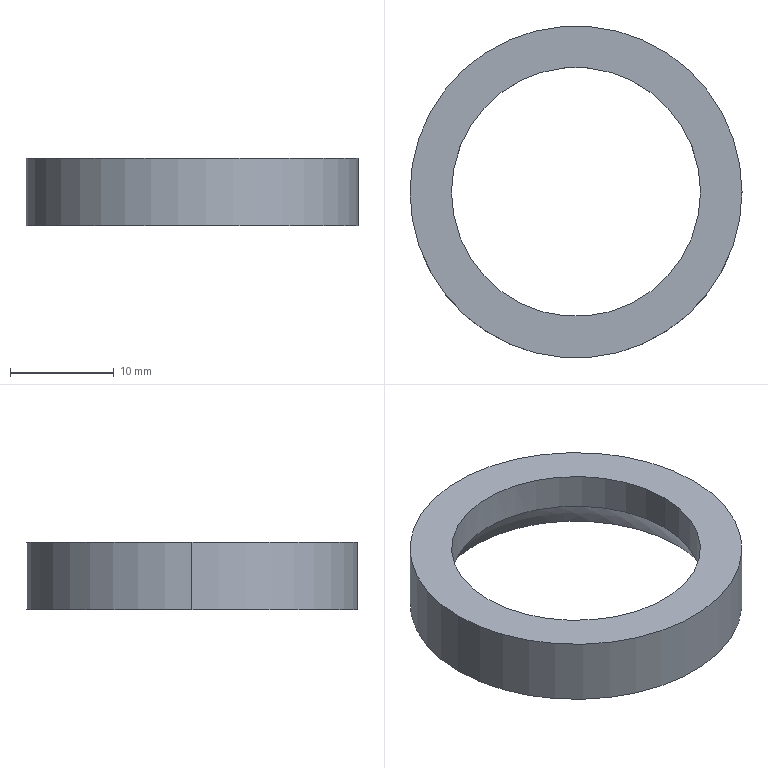Part | SolidWorks | features BaseBody 1 | 1 solid | 7 faces | box 32 x 32 x 6.5 mm | volume 2061 mm3 | cylinder 4 | plane 2 | spline 1 | commonest cylinder face diameters 24 x2 32 x2
STEP:
#1=CARTESIAN_POINT('',(16.,0.,0.));
#2=VERTEX_POINT('',#1);
#3=CARTESIAN_POINT('',(-16.,0.,0.));
#4=VERTEX_POINT('',#3);
#5=CARTESIAN_POINT('',(0.,0.,0.));
#6=DIRECTION('',(0.,0.,1.));
#7=DIRECTION('',(1.,0.,0.));
#8=AXIS2_PLACEMENT_3D('',#5,#6,#7);
#9=CIRCLE('',#8,16.);
#10=EDGE_CURVE('',#2,#4,#9,.T.);
#11=ORIENTED_EDGE('',*,*,#10,.T.);
#12=CARTESIAN_POINT('',(-16.,0.,6.5));
#13=VERTEX_POINT('',#12);
#14=CARTESIAN_POINT('',(-16.,0.,0.));
#15=DIRECTION('',(0.,0.,1.));
#16=VECTOR('',#15,1000.);
#17=LINE('',#14,#16);
#18=EDGE_CURVE('',#4,#13,#17,.T.);
#19=ORIENTED_EDGE('',*,*,#18,.T.);
#20=CARTESIAN_POINT('',(16.,0.,6.5));
#21=VERTEX_POINT('',#20);
#22=CARTESIAN_POINT('',(0.,0.,6.5));
#23=DIRECTION('',(0.,0.,-1.));
#24=DIRECTION('',(1.,0.,0.));
#25=AXIS2_PLACEMENT_3D('',#22,#23,#24);
#26=CIRCLE('',#25,16.);
#27=EDGE_CURVE('',#13,#21,#26,.T.);
#28=ORIENTED_EDGE('',*,*,#27,.T.);
#29=CARTESIAN_POINT('',(16.,0.,0.));
#30=DIRECTION('',(0.,0.,1.));
#31=VECTOR('',#30,1000.);
#32=LINE('',#29,#31);
#33=EDGE_CURVE('',#2,#21,#32,.T.);
#34=ORIENTED_EDGE('',*,*,#33,.F.);
#35=EDGE_LOOP('',(#11,#19,#28,#34));
#36=FACE_OUTER_BOUND('',#35,.T.);
#37=CARTESIAN_POINT('',(0.,0.,0.));
#38=DIRECTION('',(0.,0.,1.));
#39=DIRECTION('',(1.,0.,0.));
#40=AXIS2_PLACEMENT_3D('',#37,#38,#39);
#41=CYLINDRICAL_SURFACE('',#40,16.);
#42=ADVANCED_FACE('',(#36),#41,.T.);
#43=CARTESIAN_POINT('',(12.,0.,3.));
#44=VERTEX_POINT('',#43);
#45=CARTESIAN_POINT('',(-12.,0.,3.));
#46=VERTEX_POINT('',#45);
#47=CARTESIAN_POINT('',(0.,0.,3.));
#48=DIRECTION('',(0.,0.,-1.));
#49=DIRECTION('',(1.,0.,0.));
#50=AXIS2_PLACEMENT_3D('',#47,#48,#49);
#51=CIRCLE('',#50,12.);
#52=EDGE_CURVE('',#44,#46,#51,.T.);
#53=ORIENTED_EDGE('',*,*,#52,.T.);
#54=CARTESIAN_POINT('',(-12.,0.,6.5));
#55=VERTEX_POINT('',#54);
#56=CARTESIAN_POINT('',(-12.,0.,0.));
#57=DIRECTION('',(0.,0.,1.));
#58=VECTOR('',#57,1000.);
#59=LINE('',#56,#58);
#60=EDGE_CURVE('',#46,#55,#59,.T.);
#61=ORIENTED_EDGE('',*,*,#60,.T.);
#62=CARTESIAN_POINT('',(12.,0.,6.5));
#63=VERTEX_POINT('',#62);
#64=CARTESIAN_POINT('',(0.,0.,6.5));
#65=DIRECTION('',(0.,0.,-1.));
#66=DIRECTION('',(1.,0.,0.));
#67=AXIS2_PLACEMENT_3D('',#64,#65,#66);
#68=CIRCLE('',#67,12.);
#69=EDGE_CURVE('',#63,#55,#68,.T.);
#70=ORIENTED_EDGE('',*,*,#69,.F.);
#71=CARTESIAN_POINT('',(12.,0.,0.));
#72=DIRECTION('',(0.,0.,1.));
#73=VECTOR('',#72,1000.);
#74=LINE('',#71,#73);
#75=EDGE_CURVE('',#44,#63,#74,.T.);
#76=ORIENTED_EDGE('',*,*,#75,.F.);
#77=EDGE_LOOP('',(#53,#61,#70,#76));
#78=FACE_OUTER_BOUND('',#77,.T.);
#79=CARTESIAN_POINT('',(0.,0.,0.));
#80=DIRECTION('',(0.,0.,1.));
#81=DIRECTION('',(1.,0.,0.));
#82=AXIS2_PLACEMENT_3D('',#79,#80,#81);
#83=CYLINDRICAL_SURFACE('',#82,12.);
#84=ADVANCED_FACE('',(#78),#83,.F.);
#85=ORIENTED_EDGE('',*,*,#18,.F.);
#86=CARTESIAN_POINT('',(0.,0.,0.));
#87=DIRECTION('',(0.,0.,1.));
#88=DIRECTION('',(1.,0.,0.));
#89=AXIS2_PLACEMENT_3D('',#86,#87,#88);
#90=CIRCLE('',#89,16.);
#91=EDGE_CURVE('',#4,#2,#90,.T.);
#92=ORIENTED_EDGE('',*,*,#91,.T.);
#93=ORIENTED_EDGE('',*,*,#33,.T.);
#94=CARTESIAN_POINT('',(0.,0.,6.5));
#95=DIRECTION('',(0.,0.,-1.));
#96=DIRECTION('',(1.,0.,0.));
#97=AXIS2_PLACEMENT_3D('',#94,#95,#96);
#98=CIRCLE('',#97,16.);
#99=EDGE_CURVE('',#21,#13,#98,.T.);
#100=ORIENTED_EDGE('',*,*,#99,.T.);
#101=EDGE_LOOP('',(#85,#92,#93,#100));
#102=FACE_OUTER_BOUND('',#101,.T.);
#103=CARTESIAN_POINT('',(0.,0.,0.));
#104=DIRECTION('',(0.,0.,1.));
#105=DIRECTION('',(1.,0.,0.));
#106=AXIS2_PLACEMENT_3D('',#103,#104,#105);
#107=CYLINDRICAL_SURFACE('',#106,16.);
#108=ADVANCED_FACE('',(#102),#107,.T.);
#109=CARTESIAN_POINT('',(-13.748,0.,0.));
#110=VERTEX_POINT('',#109);
#111=CARTESIAN_POINT('',(13.748,-0.00486,0.));
#112=VERTEX_POINT('',#111);
#113=CARTESIAN_POINT('',(-13.748,0.,0.));
#114=CARTESIAN_POINT('',(-13.748,-0.9082,0.));
#115=CARTESIAN_POINT('',(-13.659,-1.801,0.));
#116=CARTESIAN_POINT('',(-13.397,-3.119,0.));
#117=CARTESIAN_POINT('',(-13.288,-3.555,0.));
#118=CARTESIAN_POINT('',(-13.026,-4.418,0.));
#119=CARTESIAN_POINT('',(-12.873,-4.848,0.));
#120=CARTESIAN_POINT('',(-12.355,-6.096,0.));
#121=CARTESIAN_POINT('',(-11.933,-6.886,0.));
#122=CARTESIAN_POINT('',(-11.185,-8.007,0.));
#123=CARTESIAN_POINT('',(-10.915,-8.371,0.));
#124=CARTESIAN_POINT('',(-10.34,-9.071,0.));
#125=CARTESIAN_POINT('',(-10.037,-9.405,0.));
#126=CARTESIAN_POINT('',(-9.086,-10.356,0.));
#127=CARTESIAN_POINT('',(-8.394,-10.925,0.));
#128=CARTESIAN_POINT('',(-7.267,-11.679,0.));
#129=CARTESIAN_POINT('',(-6.876,-11.913,0.));
#130=CARTESIAN_POINT('',(-6.083,-12.337,0.));
#131=CARTESIAN_POINT('',(-5.272,-12.72,0.));
#132=CARTESIAN_POINT('',(-4.428,-13.023,0.));
#133=CARTESIAN_POINT('',(-3.568,-13.284,0.));
#134=CARTESIAN_POINT('',(-3.127,-13.395,0.));
#135=CARTESIAN_POINT('',(-1.796,-13.66,0.));
#136=CARTESIAN_POINT('',(-0.9039,-13.747,0.));
#137=CARTESIAN_POINT('',(0.441,-13.748,0.));
#138=CARTESIAN_POINT('',(0.8904,-13.726,0.));
#139=CARTESIAN_POINT('',(1.792,-13.638,0.));
#140=CARTESIAN_POINT('',(2.241,-13.571,0.));
#141=CARTESIAN_POINT('',(3.563,-13.308,0.));
#142=CARTESIAN_POINT('',(4.42,-13.049,0.));
#143=CARTESIAN_POINT('',(5.668,-12.533,0.));
#144=CARTESIAN_POINT('',(6.08,-12.338,0.));
#145=CARTESIAN_POINT('',(6.877,-11.913,0.));
#146=CARTESIAN_POINT('',(7.262,-11.682,0.));
#147=CARTESIAN_POINT('',(8.38,-10.935,0.));
#148=CARTESIAN_POINT('',(9.074,-10.367,0.));
#149=CARTESIAN_POINT('',(10.358,-9.085,0.));
#150=CARTESIAN_POINT('',(10.928,-8.389,0.));
#151=CARTESIAN_POINT('',(11.675,-7.273,0.));
#152=CARTESIAN_POINT('',(11.906,-6.888,0.));
#153=CARTESIAN_POINT('',(12.332,-6.093,0.));
#154=CARTESIAN_POINT('',(12.527,-5.681,0.));
#155=CARTESIAN_POINT('',(13.045,-4.431,0.));
#156=CARTESIAN_POINT('',(13.305,-3.574,0.));
#157=CARTESIAN_POINT('',(13.569,-2.253,0.));
#158=CARTESIAN_POINT('',(13.636,-1.806,0.));
#159=CARTESIAN_POINT('',(13.726,-0.9034,0.));
#160=CARTESIAN_POINT('',(13.748,-0.4534,0.));
#161=CARTESIAN_POINT('',(13.748,-0.00486,0.));
#162=B_SPLINE_CURVE_WITH_KNOTS('',3,(#113,#114,#115,#116,#117,#118,#119,#120,#121,#122,#123,#124,#125,#126,#127,#128,#129,#130,#131,#132,#133,#134,#135,#136,#137,#138,#139,#140,#141,#142,#143,#144,#145,#146,#147,#148,#149,#150,#151,#152,#153,#154,#155,#156,#157,#158,#159,#160,#161),.UNSPECIFIED.,.F.,.F.,(4,2,2,2,2,2,2,2,2,1,2,2,2,2,2,2,2,2,2,2,2,2,2,2,4),(0.,0.002686,0.004029,0.005372,0.008058,0.009401,0.01074,0.01343,0.01477,0.01612,0.01746,0.0188,0.02149,0.02283,0.02417,0.02686,0.0282,0.02955,0.03223,0.03492,0.03626,0.0376,0.04029,0.04163,0.04298),.UNSPECIFIED.);
#163=EDGE_CURVE('',#110,#112,#162,.T.);
#164=ORIENTED_EDGE('',*,*,#163,.T.);
#165=CARTESIAN_POINT('',(13.748,-0.00486,0.));
#166=CARTESIAN_POINT('',(13.748,0.8923,0.));
#167=CARTESIAN_POINT('',(13.661,1.784,0.));
#168=CARTESIAN_POINT('',(13.398,3.113,0.));
#169=CARTESIAN_POINT('',(13.288,3.555,0.));
#170=CARTESIAN_POINT('',(13.027,4.417,0.));
#171=CARTESIAN_POINT('',(12.725,5.261,0.));
#172=CARTESIAN_POINT('',(12.342,6.072,0.));
#173=CARTESIAN_POINT('',(11.92,6.865,0.));
#174=CARTESIAN_POINT('',(11.687,7.255,0.));
#175=CARTESIAN_POINT('',(10.933,8.384,0.));
#176=CARTESIAN_POINT('',(10.364,9.077,0.));
#177=CARTESIAN_POINT('',(9.414,10.029,0.));
#178=CARTESIAN_POINT('',(9.081,10.331,0.));
#179=CARTESIAN_POINT('',(8.382,10.906,0.));
#180=CARTESIAN_POINT('',(8.017,11.177,0.));
#181=CARTESIAN_POINT('',(6.896,11.927,0.));
#182=CARTESIAN_POINT('',(6.107,12.35,0.));
#183=CARTESIAN_POINT('',(4.86,12.868,0.));
#184=CARTESIAN_POINT('',(4.432,13.022,0.));
#185=CARTESIAN_POINT('',(3.567,13.285,0.));
#186=CARTESIAN_POINT('',(3.131,13.394,0.));
#187=CARTESIAN_POINT('',(1.813,13.657,0.));
#188=CARTESIAN_POINT('',(0.9205,13.747,0.));
#189=CARTESIAN_POINT('',(-0.4392,13.748,0.));
#190=CARTESIAN_POINT('',(-0.8917,13.726,0.));
#191=CARTESIAN_POINT('',(-1.786,13.639,0.));
#192=CARTESIAN_POINT('',(-2.229,13.573,0.));
#193=CARTESIAN_POINT('',(-3.107,13.399,0.));
#194=CARTESIAN_POINT('',(-3.543,13.291,0.));
#195=CARTESIAN_POINT('',(-4.405,13.031,0.));
#196=CARTESIAN_POINT('',(-4.835,12.877,0.));
#197=CARTESIAN_POINT('',(-6.086,12.36,0.));
#198=CARTESIAN_POINT('',(-6.876,11.939,0.));
#199=CARTESIAN_POINT('',(-8.37,10.943,0.));
#200=CARTESIAN_POINT('',(-9.078,10.363,0.));
#201=CARTESIAN_POINT('',(-10.348,9.095,0.));
#202=CARTESIAN_POINT('',(-10.918,8.403,0.));
#203=CARTESIAN_POINT('',(-11.672,7.279,0.));
#204=CARTESIAN_POINT('',(-11.906,6.888,0.));
#205=CARTESIAN_POINT('',(-12.332,6.094,0.));
#206=CARTESIAN_POINT('',(-12.524,5.688,0.));
#207=CARTESIAN_POINT('',(-12.867,4.861,0.));
#208=CARTESIAN_POINT('',(-13.019,4.44,0.));
#209=CARTESIAN_POINT('',(-13.281,3.58,0.));
#210=CARTESIAN_POINT('',(-13.392,3.141,0.));
#211=CARTESIAN_POINT('',(-13.659,1.807,0.));
#212=CARTESIAN_POINT('',(-13.748,0.9082,0.));
#213=CARTESIAN_POINT('',(-13.748,0.,0.));
#214=B_SPLINE_CURVE_WITH_KNOTS('',3,(#165,#166,#167,#168,#169,#170,#171,#172,#173,#174,#175,#176,#177,#178,#179,#180,#181,#182,#183,#184,#185,#186,#187,#188,#189,#190,#191,#192,#193,#194,#195,#196,#197,#198,#199,#200,#201,#202,#203,#204,#205,#206,#207,#208,#209,#210,#211,#212,#213),.UNSPECIFIED.,.F.,.F.,(4,2,2,1,2,2,2,2,2,2,2,2,2,2,2,2,2,2,2,2,2,2,2,2,4),(0.04298,0.04566,0.04701,0.04835,0.04969,0.05103,0.05372,0.05506,0.05641,0.05909,0.06044,0.06178,0.06447,0.06581,0.06715,0.06849,0.06984,0.07252,0.07521,0.0779,0.07924,0.08058,0.08192,0.08327,0.08595),.UNSPECIFIED.);
#215=EDGE_CURVE('',#112,#110,#214,.T.);
#216=ORIENTED_EDGE('',*,*,#215,.T.);
#217=EDGE_LOOP('',(#164,#216));
#218=FACE_BOUND('',#217,.T.);
#219=ORIENTED_EDGE('',*,*,#10,.F.);
#220=ORIENTED_EDGE('',*,*,#91,.F.);
#221=EDGE_LOOP('',(#219,#220));
#222=FACE_OUTER_BOUND('',#221,.T.);
#223=CARTESIAN_POINT('',(0.,13.748,0.));
#224=DIRECTION('',(0.,0.,-1.));
#225=DIRECTION('',(-1.,0.,0.));
#226=AXIS2_PLACEMENT_3D('',#223,#224,#225);
#227=PLANE('',#226);
#228=ADVANCED_FACE('',(#218,#222),#227,.T.);
#229=ORIENTED_EDGE('',*,*,#99,.F.);
#230=ORIENTED_EDGE('',*,*,#27,.F.);
#231=EDGE_LOOP('',(#229,#230));
#232=FACE_OUTER_BOUND('',#231,.T.);
#233=ORIENTED_EDGE('',*,*,#69,.T.);
#234=CARTESIAN_POINT('',(0.,0.,6.5));
#235=DIRECTION('',(0.,0.,-1.));
#236=DIRECTION('',(1.,0.,0.));
#237=AXIS2_PLACEMENT_3D('',#234,#235,#236);
#238=CIRCLE('',#237,12.);
#239=EDGE_CURVE('',#55,#63,#238,.T.);
#240=ORIENTED_EDGE('',*,*,#239,.T.);
#241=EDGE_LOOP('',(#233,#240));
#242=FACE_BOUND('',#241,.T.);
#243=CARTESIAN_POINT('',(0.,16.,6.5));
#244=DIRECTION('',(0.,0.,1.));
#245=DIRECTION('',(1.,0.,0.));
#246=AXIS2_PLACEMENT_3D('',#243,#244,#245);
#247=PLANE('',#246);
#248=ADVANCED_FACE('',(#232,#242),#247,.T.);
#249=ORIENTED_EDGE('',*,*,#163,.F.);
#250=ORIENTED_EDGE('',*,*,#215,.F.);
#251=EDGE_LOOP('',(#249,#250));
#252=FACE_OUTER_BOUND('',#251,.T.);
#253=ORIENTED_EDGE('',*,*,#52,.F.);
#254=CARTESIAN_POINT('',(0.,0.,3.));
#255=DIRECTION('',(0.,0.,-1.));
#256=DIRECTION('',(1.,0.,0.));
#257=AXIS2_PLACEMENT_3D('',#254,#255,#256);
#258=CIRCLE('',#257,12.);
#259=EDGE_CURVE('',#46,#44,#258,.T.);
#260=ORIENTED_EDGE('',*,*,#259,.F.);
#261=EDGE_LOOP('',(#253,#260));
#262=FACE_BOUND('',#261,.T.);
#263=CARTESIAN_POINT('',(-5.32,13.846,-3.766));
#264=CARTESIAN_POINT('',(-2.994,13.846,1.773));
#265=CARTESIAN_POINT('',(3.012,13.846,1.766));
#266=CARTESIAN_POINT('',(5.325,13.846,-3.778));
#267=CARTESIAN_POINT('',(-18.746,7.777,1.873));
#268=CARTESIAN_POINT('',(-10.551,7.777,21.387));
#269=CARTESIAN_POINT('',(10.614,7.777,21.362));
#270=CARTESIAN_POINT('',(18.764,7.777,1.829));
#271=CARTESIAN_POINT('',(-18.667,-7.998,1.839));
#272=CARTESIAN_POINT('',(-10.506,-7.998,21.271));
#273=CARTESIAN_POINT('',(10.569,-7.998,21.246));
#274=CARTESIAN_POINT('',(18.685,-7.998,1.796));
#275=CARTESIAN_POINT('',(-5.181,-13.908,-3.824));
#276=CARTESIAN_POINT('',(-2.916,-13.908,1.568));
#277=CARTESIAN_POINT('',(2.933,-13.908,1.562));
#278=CARTESIAN_POINT('',(5.186,-13.908,-3.836));
#279=(BOUNDED_SURFACE()B_SPLINE_SURFACE(3,3,((#263,#264,#265,#266),(#267,#268,#269,#270),(#271,#272,#273,#274),(#275,#276,#277,#278)),.UNSPECIFIED.,.F.,.F.,.T.)B_SPLINE_SURFACE_WITH_KNOTS((4,4),(4,4),(0.,1.),(0.,1.),.UNSPECIFIED.)GEOMETRIC_REPRESENTATION_ITEM()RATIONAL_B_SPLINE_SURFACE(((1.,0.5908,0.5908,1.),(0.5864,0.3464,0.3464,0.5864),(0.5864,0.3464,0.3464,0.5864),(1.,0.5908,0.5908,1.)))REPRESENTATION_ITEM('')SURFACE());
#280=ADVANCED_FACE('',(#252,#262),#279,.F.);
#281=ORIENTED_EDGE('',*,*,#60,.F.);
#282=ORIENTED_EDGE('',*,*,#259,.T.);
#283=ORIENTED_EDGE('',*,*,#75,.T.);
#284=ORIENTED_EDGE('',*,*,#239,.F.);
#285=EDGE_LOOP('',(#281,#282,#283,#284));
#286=FACE_OUTER_BOUND('',#285,.T.);
#287=CARTESIAN_POINT('',(0.,0.,0.));
#288=DIRECTION('',(0.,0.,1.));
#289=DIRECTION('',(1.,0.,0.));
#290=AXIS2_PLACEMENT_3D('',#287,#288,#289);
#291=CYLINDRICAL_SURFACE('',#290,12.);
#292=ADVANCED_FACE('',(#286),#291,.F.);
#293=CLOSED_SHELL('',(#42,#84,#108,#228,#248,#280,#292));
#294=MANIFOLD_SOLID_BREP('',#293);
#295=CARTESIAN_POINT('',(0.,0.,0.));
#296=DIRECTION('',(0.,0.,1.));
#297=DIRECTION('',(1.,0.,0.));
#298=AXIS2_PLACEMENT_3D('',#295,#296,#297);
#299=(LENGTH_UNIT()NAMED_UNIT(*)SI_UNIT(.MILLI.,.METRE.));
#300=UNCERTAINTY_MEASURE_WITH_UNIT(LENGTH_MEASURE(0.00001),#299,'','');
#301=(NAMED_UNIT(*)PLANE_ANGLE_UNIT()SI_UNIT($,.RADIAN.));
#302=(NAMED_UNIT(*)SI_UNIT($,.STERADIAN.)SOLID_ANGLE_UNIT());
#303=(GEOMETRIC_REPRESENTATION_CONTEXT(3)GLOBAL_UNCERTAINTY_ASSIGNED_CONTEXT((#300))GLOBAL_UNIT_ASSIGNED_CONTEXT((#299,#301,#302))REPRESENTATION_CONTEXT('',''));
#304=ADVANCED_BREP_SHAPE_REPRESENTATION('',(#294,#298),#303);